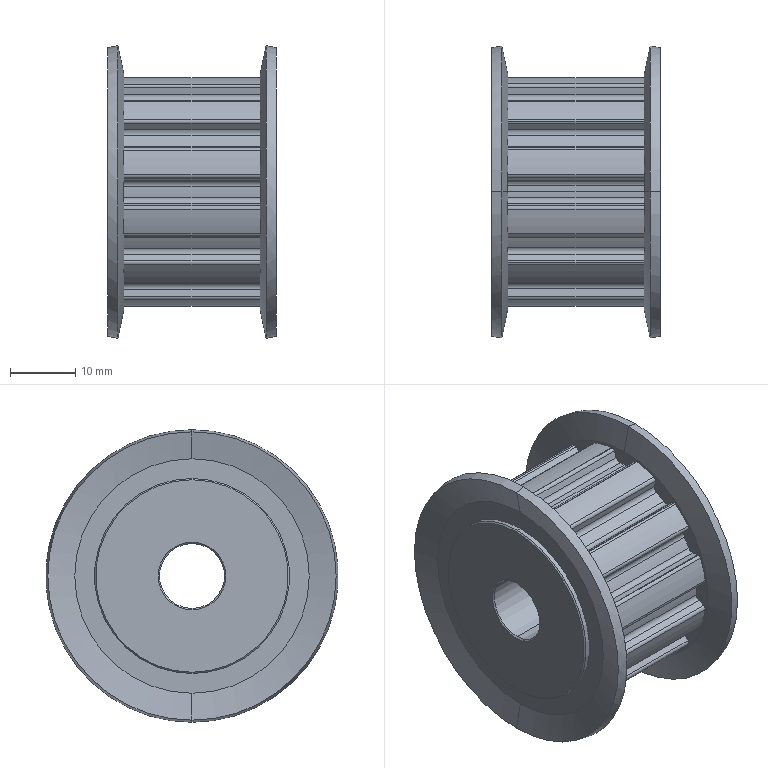Part | STEP file | ATPA12L075_A_P10_ATPA12L075-A-P10 | 1 solid | 143 faces | box 26 x 45 x 45 mm | volume 22986 mm3 | cylinder 96 | plane 31 | cone 16 | commonest cylinder face diameters 1.06 x30 1.72 x30 31.36 x14 35.62 x12 3.242 x4 30 x4